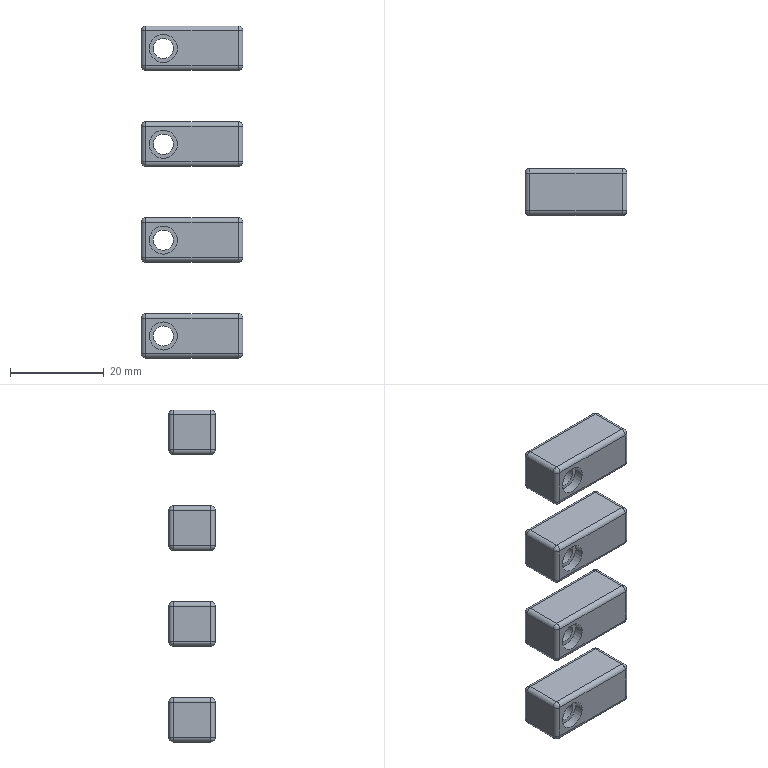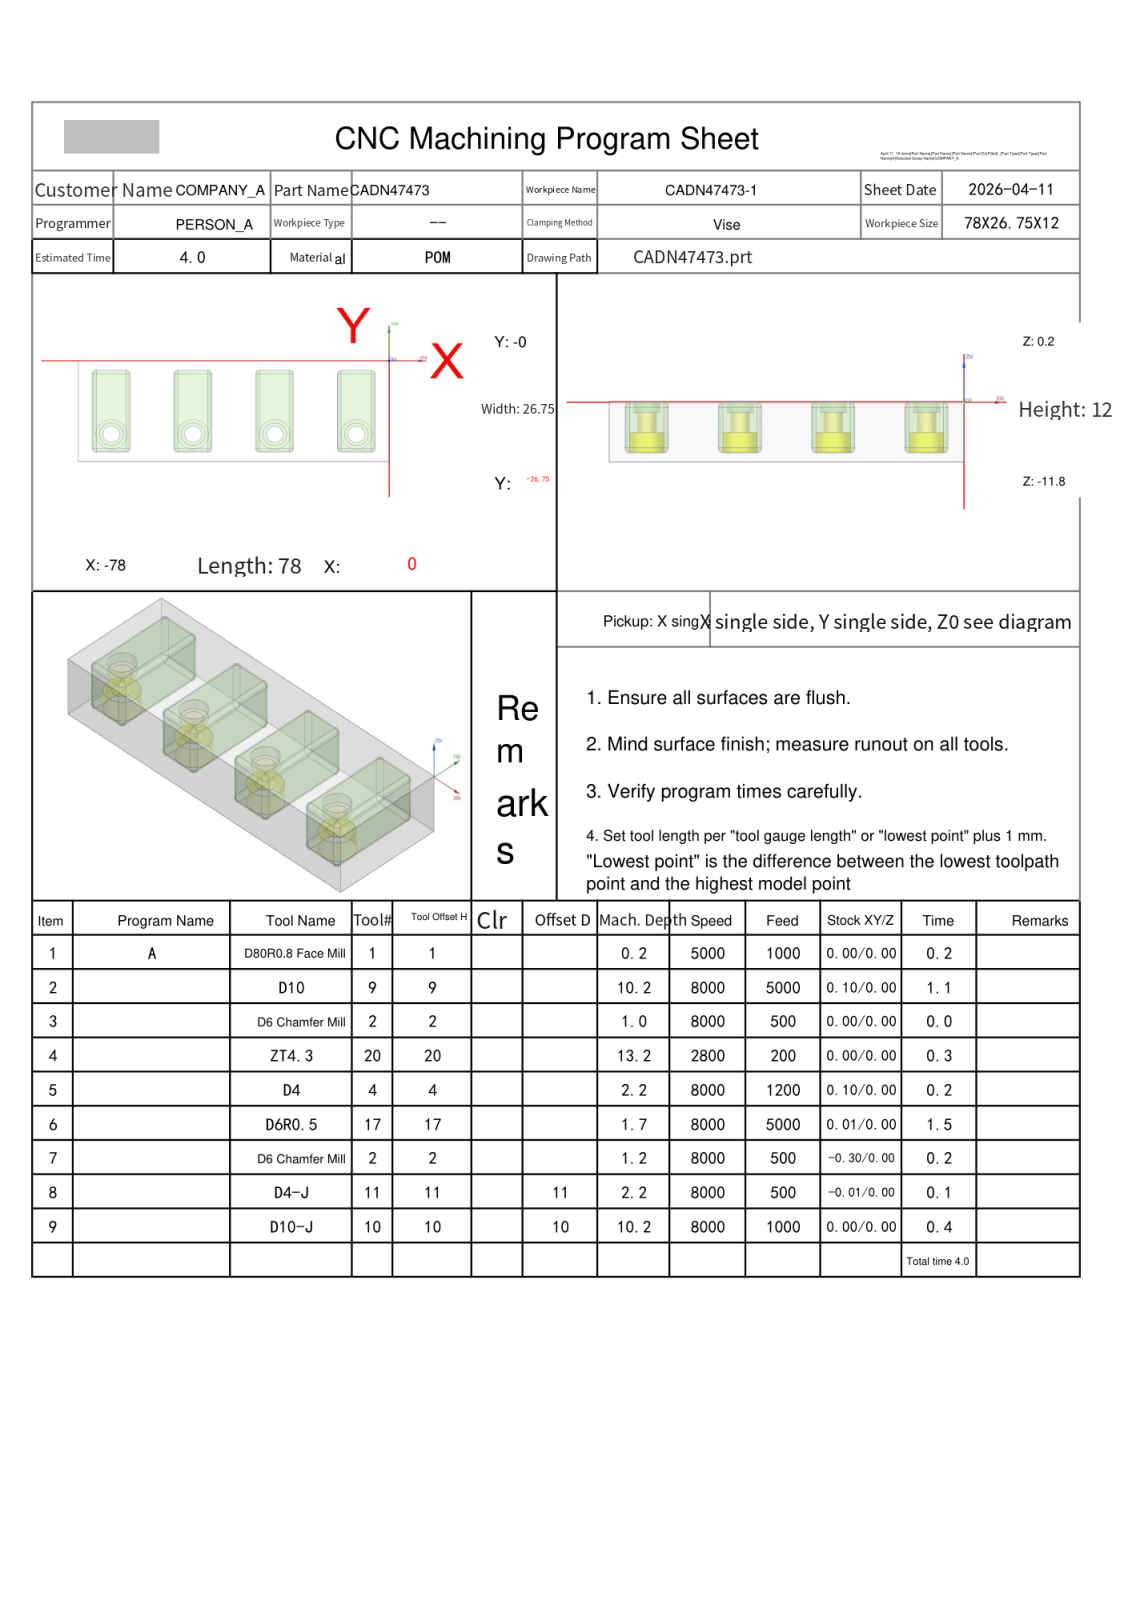NC program | NX | posted by the shop | part box 21.75 x 10 x 71 mm
Lines 681 to 1989 of 15665:
N6 T17 M06
(D6R0.5  D=6. R=0.5 H=17 ce=0.01 di=0.00)
G00 G90 G54 X-63.322 Y-10.368 M03 S8000
G43 H17 Z20.
M08
Z1.5
G01 Y-23.414 Z.816 F5000.
X-63.383 Y-23.841 Z.794
X-63.511 Y-24.253 Z.771
X-63.704 Y-24.639 Z.748
X-63.956 Y-24.989 Z.726
X-64.261 Y-25.294 Z.703
X-64.611 Y-25.546 Z.681
X-64.997 Y-25.739 Z.658
X-65.409 Y-25.867 Z.635
X-65.836 Y-25.928 Z.613
X-73.664 Z.203
X-74.091 Y-25.867 Z.18
X-74.503 Y-25.739 Z.157
X-74.889 Y-25.546 Z.135
X-75.239 Y-25.294 Z.112
X-75.544 Y-24.989 Z.09
X-75.796 Y-24.639 Z.067
X-75.989 Y-24.253 Z.044
X-76.117 Y-23.841 Z.022
X-76.178 Y-23.414 Z-.001
Y-23.25 Z-.009
Y-3.5
G02 X-73.5 Y-.822 I2.678 J0.0
G01 X-66.
G02 X-63.322 Y-3.5 I0.0 J-2.678
G01 Y-23.25
G02 X-66. Y-25.928 I-2.678 J0.0
G01 X-73.5
G02 X-76.178 Y-23.25 I0.0 J2.678
G01 X-76.181 Y-20.781 Z-.01
X-76.187 Y-18.313 Z-.011
X-76.191 Y-15.844
X-76.196 Y-13.375 Z-.012
X-76.2 Y-10.906
X-76.204 Y-8.438 Z-.013
X-76.209 Y-5.969
X-76.212 Y-3.5 Z-.014
Y-3.418
X-76.208 Y-3.336
X-76.202 Y-3.254
X-76.193 Y-3.173
X-76.183 Y-3.092
X-76.169 Y-3.011
X-76.153 Y-2.93
X-76.134 Y-2.851
X-76.114 Y-2.771
X-76.091 Y-2.693
X-76.066 Y-2.615
X-76.037 Y-2.538
X-76.008 Y-2.461
X-75.975 Y-2.386
X-75.941 Y-2.312
X-75.903 Y-2.239
X-75.865 Y-2.166
X-75.823 Y-2.096
X-75.78 Y-2.026
X-75.734 Y-1.958
X-75.687 Y-1.891
X-75.637 Y-1.826
X-75.586 Y-1.761
X-75.533 Y-1.699
X-75.478 Y-1.638
X-75.42 Y-1.58
X-75.362 Y-1.522
X-75.301 Y-1.467
X-75.239 Y-1.413
X-75.175 Y-1.362
X-75.11 Y-1.312
X-75.043 Y-1.264
X-74.975 Y-1.218
X-74.905 Y-1.175
X-74.835 Y-1.133
X-74.763 Y-1.094
X-74.69 Y-1.056
X-74.615 Y-1.022 Z-.015
X-74.54 Y-.989
X-74.464 Y-.959
X-74.387 Y-.93
X-74.309 Y-.905
X-74.23 Y-.881
X-74.15 Y-.861
X-74.071 Y-.842
X-73.99 Y-.826
X-73.909 Y-.812
X-73.828 Y-.801
X-73.746 Y-.792
X-73.664 Y-.786
X-73.582 Y-.782
X-73.5 Y-.781
X-71.625 Y-.778
X-69.75 Y-.775 Z-.016
X-67.875 Y-.772
X-66. Y-.769
X-65.918 Y-.77
X-65.835 Y-.773
X-65.753 Y-.78
X-65.671 Y-.788
X-65.589 Y-.799 Z-.017
X-65.508 Y-.813
X-65.427 Y-.829
X-65.346 Y-.847
X-65.266 Y-.868
X-65.187 Y-.891
X-65.109 Y-.917
X-65.031 Y-.945
X-64.954 Y-.975
X-64.878 Y-1.008
X-64.804 Y-1.043
X-64.73 Y-1.08
X-64.657 Y-1.119
X-64.586 Y-1.161
X-64.516 Y-1.205
X-64.447 Y-1.25
X-64.38 Y-1.298
X-64.314 Y-1.348
X-64.25 Y-1.4
X-64.187 Y-1.454
X-64.126 Y-1.509
X-64.067 Y-1.567
X-64.009 Y-1.626
X-63.953 Y-1.687
X-63.899 Y-1.749
X-63.847 Y-1.813
X-63.797 Y-1.879
X-63.749 Y-1.946
X-63.703 Y-2.015
X-63.659 Y-2.085
X-63.617 Y-2.156
X-63.578 Y-2.229
X-63.54 Y-2.302
X-63.505 Y-2.377
X-63.472 Y-2.453
X-63.442 Y-2.53
X-63.414 Y-2.607
X-63.388 Y-2.686
X-63.364 Y-2.765
X-63.343 Y-2.845
X-63.324 Y-2.926
X-63.308 Y-3.007
X-63.294 Y-3.088
X-63.283 Y-3.17
X-63.274 Y-3.252
X-63.268 Y-3.335
X-63.264 Y-3.417
X-63.263 Y-3.5
X-63.26 Y-5.969 Z-.018
X-63.256 Y-8.438
X-63.252 Y-10.906 Z-.019
X-63.249 Y-13.375 Z-.02
X-63.245 Y-15.844
X-63.243 Y-18.313 Z-.021
X-63.239 Y-20.781
X-63.236 Y-23.25 Z-.022
X-63.237 Y-23.333
X-63.241 Y-23.417
X-63.247 Y-23.5
X-63.256 Y-23.583
X-63.267 Y-23.666
X-63.28 Y-23.748
X-63.297 Y-23.83
X-63.315 Y-23.912
X-63.336 Y-23.993
X-63.36 Y-24.073
X-63.386 Y-24.152
X-63.414 Y-24.231
X-63.445 Y-24.308
X-63.478 Y-24.385
X-63.513 Y-24.461
X-63.551 Y-24.535
X-63.591 Y-24.609
X-63.633 Y-24.681
X-63.677 Y-24.752
X-63.723 Y-24.821
X-63.772 Y-24.89
X-63.822 Y-24.956
X-63.875 Y-25.021
X-63.929 Y-25.085
X-63.985 Y-25.147
X-64.043 Y-25.207
X-64.103 Y-25.265
X-64.165 Y-25.321
X-64.228 Y-25.376
X-64.293 Y-25.429
X-64.36 Y-25.479
X-64.428 Y-25.528
X-64.497 Y-25.574
X-64.568 Y-25.619
X-64.64 Y-25.661
X-64.714 Y-25.701
X-64.788 Y-25.739
X-64.864 Y-25.775
X-64.941 Y-25.808
X-65.018 Y-25.839
X-65.097 Y-25.867
X-65.176 Y-25.893 Z-.023
X-65.256 Y-25.917
X-65.337 Y-25.939
X-65.419 Y-25.957
X-65.501 Y-25.974
X-65.583 Y-25.988
X-65.666 Y-25.999
X-65.749 Y-26.008
X-65.833 Y-26.015
X-65.916 Y-26.018
X-66. Y-26.02
X-67.875 Y-26.022
X-69.75 Y-26.024 Z-.024
X-71.625 Y-26.026
X-73.5 Y-26.029
X-73.584 Y-26.028
X-73.668 Y-26.024
X-73.752 Y-26.018
X-73.835 Y-26.009
X-73.918 Y-25.998
X-74.001 Y-25.984
X-74.083 Y-25.968
X-74.165 Y-25.949
X-74.247 Y-25.928 Z-.025
X-74.327 Y-25.904
X-74.407 Y-25.878
X-74.486 Y-25.849
X-74.564 Y-25.819
X-74.641 Y-25.785
X-74.717 Y-25.75
X-74.792 Y-25.712
X-74.866 Y-25.672
X-74.938 Y-25.629
X-75.01 Y-25.585
X-75.08 Y-25.538
X-75.148 Y-25.49
X-75.215 Y-25.439
X-75.281 Y-25.387
X-75.344 Y-25.332
X-75.407 Y-25.275
X-75.467 Y-25.217
X-75.526 Y-25.157
X-75.582 Y-25.094
X-75.637 Y-25.031
X-75.69 Y-24.965
X-75.741 Y-24.899
X-75.789 Y-24.83
X-75.837 Y-24.761
X-75.881 Y-24.689
X-75.924 Y-24.617
X-75.964 Y-24.543
X-76.002 Y-24.468
X-76.037 Y-24.392
X-76.071 Y-24.315
X-76.102 Y-24.237
X-76.131 Y-24.158
X-76.157 Y-24.078
X-76.181 Y-23.997
X-76.202 Y-23.916
X-76.222 Y-23.834
X-76.238 Y-23.752
X-76.252 Y-23.669
X-76.263 Y-23.586
X-76.273 Y-23.502
X-76.279 Y-23.418
X-76.283 Y-23.334
X-76.284 Y-23.25
X-76.288 Y-20.781 Z-.026
X-76.292 Y-18.313 Z-.027
X-76.296 Y-15.844 Z-.028
X-76.3 Y-13.375
X-76.304 Y-10.906 Z-.029
X-76.308 Y-8.438 Z-.03
X-76.311 Y-5.969 Z-.031
X-76.315 Y-3.5
X-76.311 Y-3.342
X-76.298 Y-3.185 Z-.032
X-76.276 Y-3.028
X-76.245 Y-2.873
X-76.206 Y-2.72
X-76.158 Y-2.57
X-76.102 Y-2.422
X-76.038 Y-2.278
X-75.966 Y-2.137
X-75.885 Y-2.001
X-75.798 Y-1.869
X-75.703 Y-1.743
X-75.601 Y-1.622
X-75.493 Y-1.507
X-75.378 Y-1.398
X-75.257 Y-1.296
X-75.131 Y-1.201
X-75. Y-1.113
X-74.864 Y-1.032
X-74.723 Y-.96
X-74.579 Y-.895
X-74.431 Y-.838 Z-.033
X-74.281 Y-.79
X-74.128 Y-.75
X-73.973 Y-.719
X-73.816 Y-.697
X-73.658 Y-.683
X-73.5 Y-.679
X-71.625 Y-.676
X-69.75 Y-.673 Z-.034
X-67.875 Y-.67 Z-.035
X-66. Y-.667
X-65.841 Y-.672
X-65.683 Y-.685
X-65.525 Y-.707
X-65.369 Y-.737
X-65.216 Y-.777
X-65.064 Y-.825
X-64.915 Y-.882
X-64.77 Y-.946 Z-.036
X-64.629 Y-1.019
X-64.492 Y-1.1
X-64.359 Y-1.188
X-64.232 Y-1.283
X-64.111 Y-1.386
X-63.995 Y-1.495
X-63.885 Y-1.61
X-63.783 Y-1.732
X-63.687 Y-1.859
X-63.598 Y-1.991
X-63.517 Y-2.128
X-63.444 Y-2.269
X-63.379 Y-2.414
X-63.322 Y-2.563
X-63.273 Y-2.714
X-63.233 Y-2.869
X-63.202 Y-3.025
X-63.18 Y-3.182
X-63.166 Y-3.341
X-63.161 Y-3.5 Z-.037
X-63.158 Y-5.969
X-63.155 Y-8.438 Z-.038
X-63.151 Y-10.906 Z-.039
X-63.148 Y-13.375 Z-.04
X-63.145 Y-15.844
X-63.142 Y-18.313 Z-.041
X-63.139 Y-20.781 Z-.042
X-63.135 Y-23.25 Z-.043
X-63.139 Y-23.411
X-63.153 Y-23.571
X-63.175 Y-23.73
X-63.206 Y-23.888
X-63.246 Y-24.043
X-63.295 Y-24.197
X-63.352 Y-24.347
X-63.417 Y-24.494
X-63.491 Y-24.637
X-63.573 Y-24.775
X-63.662 Y-24.909
X-63.758 Y-25.038
X-63.862 Y-25.161
X-63.972 Y-25.278
X-64.089 Y-25.388
X-64.212 Y-25.492
X-64.34 Y-25.589
X-64.474 Y-25.679 Z-.044
X-64.612 Y-25.761
X-64.755 Y-25.835
X-64.902 Y-25.901
X-65.052 Y-25.958
X-65.206 Y-26.007
X-65.361 Y-26.048
X-65.519 Y-26.079
X-65.679 Y-26.102
X-65.839 Y-26.116
X-66. Y-26.121
X-67.875 Y-26.123 Z-.045
X-69.75 Y-26.125
X-71.625 Y-26.128 Z-.046
X-73.5 Y-26.13
X-73.661 Y-26.125
X-73.822 Y-26.112
X-73.982 Y-26.09 Z-.047
X-74.141 Y-26.058
X-74.298 Y-26.018
X-74.451 Y-25.969
X-74.603 Y-25.912
X-74.75 Y-25.846
X-74.894 Y-25.772
X-75.033 Y-25.69
X-75.168 Y-25.6
X-75.297 Y-25.503
X-75.421 Y-25.399
X-75.538 Y-25.288
X-75.649 Y-25.171
X-75.754 Y-25.047
X-75.851 Y-24.918
X-75.941 Y-24.784
X-76.024 Y-24.645
X-76.098 Y-24.501
X-76.164 Y-24.354
X-76.222 Y-24.202
X-76.272 Y-24.048 Z-.048
X-76.312 Y-23.892
X-76.344 Y-23.733
X-76.367 Y-23.573
X-76.381 Y-23.412
X-76.386 Y-23.25
X-76.389 Y-20.781 Z-.049
X-76.393 Y-18.313 Z-.05
X-76.396 Y-15.844 Z-.051
X-76.4 Y-13.375 Z-.052
X-76.404 Y-10.906 Z-.053
X-76.407 Y-8.438 Z-.054
X-76.41 Y-5.969 Z-.055
X-76.414 Y-3.5 Z-.056
X-76.41 Y-3.337
X-76.396 Y-3.174
X-76.374 Y-3.012
X-76.342 Y-2.851
X-76.301 Y-2.693
X-76.252 Y-2.537
X-76.194 Y-2.384
X-76.127 Y-2.235
X-76.052 Y-2.089
X-75.969 Y-1.948
X-75.879 Y-1.812
X-75.78 Y-1.681
X-75.675 Y-1.556
X-75.563 Y-1.437
X-75.444 Y-1.324 Z-.057
X-75.319 Y-1.219
X-75.189 Y-1.12
X-75.053 Y-1.029
X-74.912 Y-.946
X-74.766 Y-.87
X-74.617 Y-.803
X-74.464 Y-.745
X-74.308 Y-.695
X-74.15 Y-.654
X-73.989 Y-.621
X-73.827 Y-.598
X-73.664 Y-.584
X-73.5 Y-.58
X-71.625 Y-.577 Z-.058
X-69.75 Y-.574 Z-.059
X-67.875 Y-.572 Z-.06
X-66. Y-.569
X-65.836 Y-.573
X-65.672 Y-.587
X-65.509 Y-.61 Z-.061
X-65.348 Y-.642
X-65.188 Y-.683
X-65.031 Y-.732
X-64.878 Y-.791
X-64.727 Y-.858
X-64.581 Y-.933
X-64.439 Y-1.016
X-64.303 Y-1.108
X-64.171 Y-1.206
X-64.045 Y-1.312
X-63.925 Y-1.425
X-63.812 Y-1.545
X-63.706 Y-1.67
X-63.607 Y-1.802
X-63.515 Y-1.938 Z-.062
X-63.431 Y-2.08
X-63.355 Y-2.226
X-63.288 Y-2.377
X-63.229 Y-2.53
X-63.179 Y-2.687
X-63.137 Y-2.847
X-63.105 Y-3.008
X-63.082 Y-3.171
X-63.068 Y-3.335
X-63.063 Y-3.5
X-63.059 Y-5.969 Z-.063
X-63.056 Y-8.438 Z-.064
X-63.053 Y-10.906 Z-.065
X-63.05 Y-13.375 Z-.066
X-63.047 Y-15.844 Z-.067
X-63.044 Y-18.313 Z-.068
X-63.041 Y-20.781 Z-.069
X-63.038 Y-23.25 Z-.07
X-63.042 Y-23.416
X-63.056 Y-23.582
X-63.079 Y-23.746
X-63.111 Y-23.909
X-63.152 Y-24.07
X-63.203 Y-24.229
X-63.262 Y-24.384
X-63.329 Y-24.536
X-63.405 Y-24.684 Z-.071
X-63.49 Y-24.827
X-63.582 Y-24.966
X-63.682 Y-25.099
X-63.789 Y-25.226
X-63.903 Y-25.347
X-64.024 Y-25.461
X-64.151 Y-25.569
X-64.284 Y-25.669
X-64.422 Y-25.762
X-64.565 Y-25.846
X-64.713 Y-25.923
X-64.865 Y-25.991
X-65.02 Y-26.051
X-65.179 Y-26.101
X-65.34 Y-26.143 Z-.072
X-65.503 Y-26.176
X-65.668 Y-26.199
X-65.834 Y-26.213
X-66. Y-26.218
X-67.875 Y-26.22 Z-.073
X-69.75 Y-26.223
X-71.625 Y-26.225 Z-.074
X-73.5 Y-26.227 Z-.075
X-73.667 Y-26.223
X-73.833 Y-26.209
X-73.999 Y-26.186
X-74.163 Y-26.154
X-74.325 Y-26.112
X-74.484 Y-26.061
X-74.64 Y-26.002
X-74.793 Y-25.934
X-74.941 Y-25.858
X-75.085 Y-25.773
X-75.224 Y-25.68
X-75.358 Y-25.58 Z-.076
X-75.486 Y-25.472
X-75.607 Y-25.357
X-75.722 Y-25.236
X-75.83 Y-25.108
X-75.931 Y-24.975
X-76.024 Y-24.836
X-76.109 Y-24.692
X-76.186 Y-24.544
X-76.255 Y-24.391
X-76.314 Y-24.235
X-76.366 Y-24.076
X-76.407 Y-23.914
X-76.44 Y-23.75
X-76.464 Y-23.584
X-76.478 Y-23.417 Z-.077
X-76.483 Y-23.25
X-76.487 Y-20.781 Z-.078
X-76.49 Y-18.313 Z-.079
X-76.494 Y-15.844 Z-.08
X-76.497 Y-13.375 Z-.081
X-76.501 Y-10.906 Z-.083
X-76.504 Y-8.438 Z-.084
X-76.507 Y-5.969 Z-.085
X-76.51 Y-3.5 Z-.086
X-76.506 Y-3.331
X-76.492 Y-3.163
X-76.469 Y-2.996
X-76.436 Y-2.83
X-76.394 Y-2.666
X-76.343 Y-2.505 Z-.087
X-76.283 Y-2.347
X-76.214 Y-2.193
X-76.137 Y-2.043
X-76.051 Y-1.897
X-75.957 Y-1.756
X-75.856 Y-1.621
X-75.747 Y-1.492
X-75.631 Y-1.369
X-75.508 Y-1.253
X-75.379 Y-1.144
X-75.244 Y-1.042
X-75.104 Y-.948 Z-.088
X-74.958 Y-.861
X-74.808 Y-.784
X-74.654 Y-.714
X-74.496 Y-.654
X-74.335 Y-.602
X-74.171 Y-.56
X-74.005 Y-.526
X-73.838 Y-.503
X-73.669 Y-.488
X-73.5 Y-.483
X-71.625 Y-.481 Z-.089
X-69.75 Y-.478 Z-.09
X-67.875 Y-.476 Z-.091
X-66. Y-.473 Z-.092
X-65.83 Y-.478
X-65.661 Y-.492
X-65.493 Y-.515
X-65.326 Y-.548
X-65.162 Y-.59
X-65. Y-.642
X-64.841 Y-.702
X-64.686 Y-.771 Z-.093
X-64.535 Y-.849
X-64.388 Y-.935
X-64.247 Y-1.03
X-64.111 Y-1.131
X-63.981 Y-1.241
X-63.857 Y-1.357
X-63.741 Y-1.481
X-63.631 Y-1.611
X-63.528 Y-1.746
X-63.434 Y-1.887
X-63.347 Y-2.034
X-63.269 Y-2.185 Z-.094
X-63.199 Y-2.34
X-63.138 Y-2.499
X-63.087 Y-2.661
X-63.044 Y-2.825
X-63.011 Y-2.992
X-62.986 Y-3.16
X-62.972 Y-3.33
X-62.967 Y-3.5
X-62.964 Y-5.969 Z-.095
X-62.961 Y-8.438 Z-.097
X-62.958 Y-10.906 Z-.098
X-62.955 Y-13.375 Z-.099
X-62.951 Y-15.844 Z-.1
X-62.949 Y-18.313 Z-.101
X-62.946 Y-20.781 Z-.102
X-62.942 Y-23.25 Z-.104
X-62.947 Y-23.421
X-62.961 Y-23.592
X-62.985 Y-23.762
X-63.018 Y-23.931
X-63.061 Y-24.097
X-63.113 Y-24.26
X-63.174 Y-24.421
X-63.244 Y-24.577
X-63.322 Y-24.73
X-63.409 Y-24.878
X-63.504 Y-25.021 Z-.105
X-63.608 Y-25.158
X-63.718 Y-25.289
X-63.836 Y-25.414
X-63.961 Y-25.532
X-64.092 Y-25.643
X-64.229 Y-25.747
X-64.371 Y-25.842
X-64.519 Y-25.93
X-64.672 Y-26.009
X-64.828 Y-26.079
X-64.989 Y-26.14
X-65.152 Y-26.193
X-65.319 Y-26.236 Z-.106
X-65.487 Y-26.27
X-65.657 Y-26.294
X-65.828 Y-26.308
X-66. Y-26.313
X-67.875 Y-26.316 Z-.107
X-69.75 Y-26.318 Z-.108
X-71.625 Y-26.32 Z-.109
X-73.5 Y-26.322
X-73.672 Y-26.318 Z-.11
X-73.844 Y-26.303
X-74.015 Y-26.28
X-74.184 Y-26.246
X-74.351 Y-26.203
X-74.515 Y-26.151
X-74.676 Y-26.09
X-74.834 Y-26.02
X-74.987 Y-25.941
X-75.136 Y-25.853
X-75.279 Y-25.758
X-75.417 Y-25.654
X-75.549 Y-25.543 Z-.111
X-75.674 Y-25.424
X-75.793 Y-25.299
X-75.905 Y-25.168
X-76.009 Y-25.03
X-76.104 Y-24.887
X-76.192 Y-24.738
X-76.272 Y-24.585
X-76.342 Y-24.427
X-76.404 Y-24.266
X-76.457 Y-24.102
X-76.5 Y-23.935
X-76.534 Y-23.765 Z-.112
X-76.558 Y-23.595
X-76.573 Y-23.423
X-76.578 Y-23.25
X-76.582 Y-20.781 Z-.113
X-76.585 Y-18.313 Z-.115
X-76.588 Y-15.844 Z-.116
X-76.591 Y-13.375 Z-.117
X-76.595 Y-10.906 Z-.119
X-76.598 Y-8.438 Z-.12
X-76.601 Y-5.969 Z-.121
X-76.604 Y-3.5 Z-.123
X-76.603 Y-3.413
X-76.6 Y-3.326
X-76.594 Y-3.239
X-76.585 Y-3.152
X-76.574 Y-3.066
X-76.561 Y-2.98
X-76.545 Y-2.894
X-76.527 Y-2.809
X-76.507 Y-2.724
X-76.484 Y-2.64
X-76.459 Y-2.557
X-76.431 Y-2.474
X-76.401 Y-2.392
X-76.369 Y-2.311
X-76.335 Y-2.231 Z-.124
X-76.298 Y-2.152
X-76.26 Y-2.074
X-76.219 Y-1.997
X-76.176 Y-1.922
X-76.13 Y-1.847
X-76.083 Y-1.774
X-76.034 Y-1.702
X-75.982 Y-1.632
X-75.929 Y-1.563
X-75.874 Y-1.495
X-75.817 Y-1.43
X-75.758 Y-1.365
X-75.697 Y-1.303
X-75.635 Y-1.242
X-75.571 Y-1.183
X-75.505 Y-1.126
X-75.438 Y-1.07
X-75.369 Y-1.017
X-75.298 Y-.965
X-75.227 Y-.916
X-75.154 Y-.868 Z-.125
X-75.079 Y-.823
X-75.004 Y-.779
X-74.927 Y-.738
X-74.849 Y-.699
X-74.77 Y-.662
X-74.69 Y-.628
X-74.609 Y-.595
X-74.527 Y-.565
X-74.444 Y-.538
X-74.361 Y-.512
X-74.277 Y-.489
X-74.192 Y-.469
X-74.107 Y-.45
X-74.021 Y-.434
X-73.935 Y-.421
X-73.848 Y-.41
X-73.761 Y-.401
X-73.674 Y-.395
X-73.587 Y-.391
X-73.5 Y-.39 Z-.126
X-71.625 Y-.387 Z-.127
X-69.75 Y-.385 Z-.128
X-67.875 Y-.383 Z-.129
X-66. Y-.38 Z-.13
X-65.825 Y-.385
X-65.651 Y-.399
X-65.477 Y-.424
X-65.306 Y-.457
X-65.136 Y-.501
X-64.969 Y-.554
X-64.805 Y-.616
X-64.646 Y-.687
X-64.49 Y-.768 Z-.131
X-64.339 Y-.856
X-64.193 Y-.954
X-64.053 Y-1.059
X-63.919 Y-1.172
X-63.792 Y-1.292
X-63.671 Y-1.419
X-63.558 Y-1.552
X-63.452 Y-1.692
X-63.355 Y-1.838
X-63.266 Y-1.989 Z-.132
X-63.185 Y-2.144
X-63.113 Y-2.304
X-63.05 Y-2.468
X-62.997 Y-2.635
X-62.953 Y-2.805
X-62.919 Y-2.976
X-62.894 Y-3.15
X-62.879 Y-3.325
X-62.874 Y-3.5
X-62.871 Y-5.969 Z-.134
X-62.868 Y-8.438 Z-.135
X-62.865 Y-10.906 Z-.137
X-62.862 Y-13.375 Z-.138
X-62.859 Y-15.844 Z-.139
X-62.856 Y-18.313 Z-.141
X-62.853 Y-20.781 Z-.142
X-62.85 Y-23.25 Z-.143
X-62.851 Y-23.338
X-62.855 Y-23.427 Z-.144
X-62.861 Y-23.515
X-62.87 Y-23.603
X-62.881 Y-23.69
X-62.894 Y-23.778
X-62.91 Y-23.865
X-62.928 Y-23.951
X-62.949 Y-24.037
X-62.972 Y-24.122
X-62.998 Y-24.207
X-63.026 Y-24.291
X-63.089 Y-24.456
X-63.161 Y-24.617
X-63.242 Y-24.775
X-63.331 Y-24.927
X-63.429 Y-25.074
X-63.535 Y-25.215 Z-.145
X-63.649 Y-25.351
X-63.771 Y-25.479
X-63.899 Y-25.601
X-64.034 Y-25.715
X-64.175 Y-25.822
X-64.322 Y-25.92
X-64.474 Y-26.01
X-64.632 Y-26.092
X-64.793 Y-26.164
X-64.958 Y-26.227 Z-.146
X-65.127 Y-26.281
X-65.298 Y-26.326
X-65.472 Y-26.36
X-65.647 Y-26.385
X-65.823 Y-26.401
X-66. Y-26.406
X-67.875 Y-26.408 Z-.147
X-69.75 Y-26.41 Z-.148
X-71.625 Y-26.412 Z-.149
X-73.5 Y-26.414 Z-.15
X-73.677 Y-26.41
X-73.854 Y-26.395 Z-.151
X-74.03 Y-26.37
X-74.204 Y-26.336
X-74.376 Y-26.292
X-74.546 Y-26.238
X-74.712 Y-26.175
X-74.874 Y-26.102
X-75.032 Y-26.021
X-75.185 Y-25.931
X-75.332 Y-25.833
X-75.474 Y-25.726 Z-.152
X-75.61 Y-25.611
X-75.74 Y-25.49
X-75.862 Y-25.361
X-75.977 Y-25.225
X-76.084 Y-25.083
X-76.182 Y-24.935
X-76.273 Y-24.783
X-76.355 Y-24.625
X-76.392 Y-24.544
X-76.427 Y-24.463
X-76.46 Y-24.38
X-76.491 Y-24.297 Z-.153
X-76.519 Y-24.212
X-76.545 Y-24.127
X-76.569 Y-24.042
X-76.59 Y-23.955
X-76.608 Y-23.868
X-76.625 Y-23.781
X-76.638 Y-23.693
X-76.65 Y-23.605
X-76.665 Y-23.428
X-76.67 Y-23.25
X-76.673 Y-20.781 Z-.155
X-76.677 Y-18.313 Z-.156
X-76.68 Y-15.844 Z-.158
X-76.683 Y-13.375 Z-.159
X-76.686 Y-10.906 Z-.161
X-76.689 Y-8.438 Z-.162
X-76.692 Y-5.969 Z-.164
X-76.695 Y-3.5 Z-.166
X-76.694 Y-3.41
X-76.69 Y-3.321
X-76.684 Y-3.231
X-76.675 Y-3.142
X-76.664 Y-3.053
X-76.65 Y-2.965
X-76.634 Y-2.877
X-76.616 Y-2.789
X-76.595 Y-2.702
X-76.571 Y-2.615
X-76.545 Y-2.529
X-76.517 Y-2.444
X-76.486 Y-2.36
X-76.453 Y-2.277
X-76.418 Y-2.194
X-76.38 Y-2.113 Z-.167
X-76.34 Y-2.033
X-76.298 Y-1.954
X-76.254 Y-1.876
X-76.207 Y-1.799
X-76.159 Y-1.724
X-76.108 Y-1.65
X-76.055 Y-1.577
X-76. Y-1.506
X-75.943 Y-1.437
X-75.884 Y-1.369
X-75.824 Y-1.303
X-75.761 Y-1.239
X-75.697 Y-1.176
X-75.631 Y-1.115
X-75.564 Y-1.056
X-75.494 Y-.999
X-75.423 Y-.944
X-75.351 Y-.891 Z-.168
X-75.277 Y-.84
X-75.202 Y-.791
X-75.125 Y-.745
X-75.047 Y-.7
X-74.968 Y-.658
X-74.888 Y-.618
X-74.807 Y-.579
X-74.724 Y-.544
X-74.641 Y-.511
X-74.557 Y-.48
X-74.472 Y-.451
X-74.386 Y-.425
X-74.299 Y-.401
X-74.212 Y-.38
X-74.124 Y-.361
X-74.036 Y-.345
X-73.947 Y-.331 Z-.169
X-73.858 Y-.32
X-73.769 Y-.31
X-73.679 Y-.304
X-73.59 Y-.3
X-73.5 Y-.299
X-71.625 Y-.296 Z-.17
X-69.75 Y-.294 Z-.171
X-67.875 Y-.292 Z-.172
X-66. Y-.29 Z-.174
X-65.91 Y-.291
X-65.82 Y-.295
X-65.73 Y-.301
X-65.641 Y-.31
X-65.551 Y-.321
X-65.462 Y-.334
X-65.374 Y-.351
X-65.285 Y-.369
X-65.198 Y-.391
X-65.111 Y-.414
X-65.025 Y-.44
X-64.939 Y-.469
X-64.855 Y-.499
X-64.771 Y-.533
X-64.688 Y-.568
X-64.606 Y-.606
X-64.526 Y-.646 Z-.175
X-64.446 Y-.689
X-64.368 Y-.733
X-64.291 Y-.78
X-64.215 Y-.829
X-64.141 Y-.88
X-64.068 Y-.933
X-63.997 Y-.988
X-63.927 Y-1.045
X-63.859 Y-1.104
X-63.793 Y-1.165
X-63.728 Y-1.228
X-63.665 Y-1.292
X-63.604 Y-1.359
X-63.545 Y-1.427
X-63.487 Y-1.496
X-63.432 Y-1.567
X-63.379 Y-1.64
X-63.328 Y-1.714 Z-.176
X-63.278 Y-1.79
X-63.232 Y-1.867
X-63.187 Y-1.945
X-63.144 Y-2.025
X-63.104 Y-2.105
X-63.066 Y-2.187
X-63.03 Y-2.27
X-62.996 Y-2.353
X-62.965 Y-2.438
X-62.937 Y-2.524
X-62.91 Y-2.61
X-62.887 Y-2.697
X-62.865 Y-2.784
X-62.846 Y-2.873
X-62.83 Y-2.961
X-62.816 Y-3.05
X-62.804 Y-3.14
X-62.795 Y-3.23 Z-.177
X-62.789 Y-3.32
X-62.785 Y-3.41
X-62.784 Y-3.5
X-62.781 Y-5.969 Z-.178
X-62.778 Y-8.438 Z-.18
X-62.775 Y-10.906 Z-.181
X-62.772 Y-13.375 Z-.183
X-62.769 Y-15.844 Z-.185
X-62.767 Y-18.313 Z-.186
X-62.764 Y-20.781 Z-.188
X-62.761 Y-23.25 Z-.189
X-62.762 Y-23.341
X-62.766 Y-23.432
X-62.772 Y-23.522
X-62.781 Y-23.613
X-62.792 Y-23.703 Z-.19
X-62.806 Y-23.793
X-62.822 Y-23.882
X-62.841 Y-23.971
X-62.863 Y-24.059
X-62.887 Y-24.147
X-62.913 Y-24.234
X-62.942 Y-24.32
X-62.973 Y-24.406
X-63.006 Y-24.49
X-63.042 Y-24.574
X-63.08 Y-24.656
X-63.121 Y-24.738
X-63.163 Y-24.818
X-63.208 Y-24.897
X-63.256 Y-24.974
X-63.305 Y-25.051
X-63.356 Y-25.126
X-63.41 Y-25.199 Z-.191
X-63.466 Y-25.271
X-63.523 Y-25.342
X-63.583 Y-25.41
X-63.644 Y-25.477
X-63.708 Y-25.542
X-63.773 Y-25.606
X-63.84 Y-25.667
X-63.908 Y-25.727
X-63.978 Y-25.785
X-64.05 Y-25.841
X-64.124 Y-25.895
X-64.198 Y-25.946
X-64.275 Y-25.996
X-64.352 Y-26.043
X-64.431 Y-26.088
X-64.511 Y-26.131
X-64.593 Y-26.172 Z-.192
X-64.675 Y-26.211
X-64.759 Y-26.247
X-64.843 Y-26.28
X-64.929 Y-26.312
X-65.015 Y-26.341
X-65.102 Y-26.367
X-65.19 Y-26.391
X-65.278 Y-26.413
X-65.367 Y-26.432
X-65.457 Y-26.448
X-65.546 Y-26.463
X-65.637 Y-26.474
X-65.727 Y-26.483
X-65.818 Y-26.49
X-65.909 Y-26.494
X-66. Y-26.495
X-67.875 Y-26.497 Z-.194
X-69.75 Y-26.499 Z-.195
X-71.625 Y-26.501 Z-.196
X-73.5 Y-26.503 Z-.197
X-73.591 Y-26.502
X-73.682 Y-26.498
X-73.773 Y-26.492
X-73.864 Y-26.483
X-73.955 Y-26.472
X-74.045 Y-26.458 Z-.198
X-74.135 Y-26.442
X-74.224 Y-26.423
X-74.313 Y-26.401
X-74.401 Y-26.377
X-74.488 Y-26.351
X-74.575 Y-26.322
X-74.661 Y-26.291
X-74.746 Y-26.257
X-74.829 Y-26.221
X-74.912 Y-26.183
X-74.994 Y-26.142
X-75.075 Y-26.099
X-75.154 Y-26.054
X-75.232 Y-26.006
X-75.309 Y-25.957
X-75.384 Y-25.905
X-75.458 Y-25.851 Z-.199
X-75.53 Y-25.795
X-75.601 Y-25.738
X-75.67 Y-25.678
X-75.737 Y-25.616
X-75.802 Y-25.552
X-75.866 Y-25.487
X-75.928 Y-25.42
X-75.988 Y-25.351
X-76.046 Y-25.28
X-76.102 Y-25.208
X-76.156 Y-25.135
X-76.208 Y-25.059
X-76.258 Y-24.983
X-76.305 Y-24.905
X-76.351 Y-24.826
X-76.394 Y-24.745
X-76.435 Y-24.663
X-76.473 Y-24.581 Z-.2
X-76.51 Y-24.497
X-76.544 Y-24.412
X-76.575 Y-24.326
X-76.604 Y-24.239
X-76.631 Y-24.152
X-76.655 Y-24.064
X-76.676 Y-23.975
X-76.696 Y-23.886
X-76.712 Y-23.796
X-76.727 Y-23.706
X-76.738 Y-23.615
X-76.747 Y-23.524
X-76.754 Y-23.433
X-76.758 Y-23.341
X-76.759 Y-23.25
X-76.762 Y-20.781 Z-.202
X-76.765 Y-18.313 Z-.204
X-76.768 Y-15.844 Z-.206
X-76.771 Y-13.375 Z-.207
X-76.774 Y-10.906 Z-.209
X-76.777 Y-8.438 Z-.211
X-76.779 Y-5.969 Z-.213
X-76.782 Y-3.5 Z-.214
X-76.778 Y-3.328
X-76.765 Y-3.157 Z-.215
X-76.743 Y-2.986
X-76.711 Y-2.817
X-76.672 Y-2.65
X-76.623 Y-2.485
X-76.566 Y-2.323
X-76.5 Y-2.164
X-76.426 Y-2.009
X-76.344 Y-1.858 Z-.216
X-76.255 Y-1.711
X-76.157 Y-1.569
X-76.053 Y-1.433
X-75.941 Y-1.302
X-75.823 Y-1.177
X-75.699 Y-1.058
X-75.568 Y-.946
X-75.431 Y-.842 Z-.217
X-75.29 Y-.744
X-75.143 Y-.654
X-74.992 Y-.571
X-74.837 Y-.497
X-74.678 Y-.431
X-74.516 Y-.374
X-74.351 Y-.324
X-74.184 Y-.284
X-74.014 Y-.253 Z-.218
X-73.844 Y-.23
X-73.672 Y-.216
X-73.5 Y-.212
X-71.625 Y-.209 Z-.219
X-69.75 Y-.207 Z-.221
X-67.875 Y-.205 Z-.222
X-66. Y-.203 Z-.223
X-65.827 Y-.207
X-65.655 Y-.22 Z-.224
X-65.484 Y-.243
X-65.314 Y-.274
X-65.146 Y-.314
X-64.981 Y-.363
X-64.818 Y-.421
X-64.658 Y-.486
X-64.502 Y-.561
X-64.35 Y-.643
X-64.203 Y-.733 Z-.225
X-64.061 Y-.831
X-63.923 Y-.936
X-63.792 Y-1.048
X-63.666 Y-1.166
X-63.547 Y-1.292
X-63.435 Y-1.423
X-63.33 Y-1.56
X-63.232 Y-1.702 Z-.226
X-63.141 Y-1.849
X-63.058 Y-2.001
X-62.984 Y-2.157
X-62.918 Y-2.317
X-62.86 Y-2.48
X-62.81 Y-2.645
X-62.77 Y-2.813
X-62.738 Y-2.983 Z-.227
X-62.715 Y-3.155
X-62.702 Y-3.327
X-62.697 Y-3.5
X-62.694 Y-5.969 Z-.229
X-62.691 Y-8.438 Z-.23
X-62.689 Y-10.906 Z-.232
X-62.686 Y-13.375 Z-.234
X-62.683 Y-15.844 Z-.236
X-62.681 Y-18.313 Z-.237
X-62.678 Y-20.781 Z-.239
X-62.675 Y-23.25 Z-.241
X-62.679 Y-23.424
X-62.693 Y-23.598
X-62.715 Y-23.77
X-62.747 Y-23.941
X-62.787 Y-24.111
X-62.837 Y-24.278 Z-.242
X-62.895 Y-24.442
X-62.961 Y-24.603
X-63.036 Y-24.76
X-63.119 Y-24.913
X-63.21 Y-25.062
X-63.308 Y-25.206
X-63.414 Y-25.344
X-63.527 Y-25.477 Z-.243
X-63.647 Y-25.603
X-63.773 Y-25.723
X-63.906 Y-25.837
X-64.044 Y-25.943
X-64.187 Y-26.042
X-64.336 Y-26.133
X-64.489 Y-26.216
X-64.646 Y-26.291 Z-.244
X-64.807 Y-26.358
X-64.971 Y-26.417
X-65.138 Y-26.466
X-65.308 Y-26.507
X-65.479 Y-26.539
X-65.652 Y-26.562
X-65.826 Y-26.576
X-66. Y-26.581 Z-.245
X-67.875 Y-26.583 Z-.246
X-69.75 Y-26.585 Z-.247
X-71.625 Y-26.587 Z-.248
X-73.5 Y-26.589 Z-.25
X-73.675 Y-26.584
X-73.849 Y-26.571
X-74.022 Y-26.548
X-74.194 Y-26.517
X-74.364 Y-26.476
X-74.532 Y-26.426 Z-.251
X-74.697 Y-26.368
X-74.859 Y-26.301
X-75.016 Y-26.226
X-75.17 Y-26.143
X-75.319 Y-26.052
X-75.464 Y-25.953
X-75.603 Y-25.847
X-75.736 Y-25.733 Z-.252
X-75.863 Y-25.613
X-75.983 Y-25.486
X-76.097 Y-25.353
X-76.204 Y-25.214
X-76.303 Y-25.07
X-76.395 Y-24.921
X-76.478 Y-24.767
X-76.554 Y-24.61 Z-.253
X-76.621 Y-24.448
X-76.68 Y-24.283
X-76.729 Y-24.115
X-76.77 Y-23.945
X-76.803 Y-23.773
X-76.826 Y-23.6
X-76.839 Y-23.425
X-76.844 Y-23.25
X-76.847 Y-20.781 Z-.255
X-76.85 Y-18.313 Z-.257
X-76.852 Y-15.844 Z-.259
X-76.856 Y-13.375 Z-.261
X-76.858 Y-10.906 Z-.263
X-76.861 Y-8.438 Z-.265
X-76.864 Y-5.969 Z-.267
X-76.866 Y-3.5 Z-.269
X-76.862 Y-3.324
X-76.848 Y-3.148
X-76.826 Y-2.973
X-76.794 Y-2.8
X-76.753 Y-2.628
X-76.703 Y-2.459 Z-.27
X-76.644 Y-2.293
X-76.577 Y-2.13
X-76.501 Y-1.971
X-76.417 Y-1.816
X-76.325 Y-1.665
X-76.225 Y-1.52
X-76.118 Y-1.38 Z-.271
X-76.004 Y-1.246
X-75.883 Y-1.117
X-75.755 Y-.996
X-75.621 Y-.881
X-75.481 Y-.774
X-75.336 Y-.673
X-75.185 Y-.581
X-75.03 Y-.497 Z-.272
X-74.871 Y-.421
X-74.708 Y-.353
X-74.542 Y-.294
X-74.373 Y-.243
X-74.201 Y-.202
X-74.027 Y-.17
X-73.852 Y-.147 Z-.273
X-73.676 Y-.132
X-73.5 Y-.128
X-71.625 Y-.126 Z-.274
X-69.75 Y-.123 Z-.276
X-67.875 Y-.121 Z-.277
X-66. Y-.119 Z-.279
X-65.823 Y-.124
X-65.647 Y-.137
X-65.471 Y-.16
X-65.297 Y-.192
X-65.125 Y-.234
X-64.955 Y-.284
X-64.788 Y-.343 Z-.28
X-64.624 Y-.41
X-64.464 Y-.486
X-64.309 Y-.571
X-64.158 Y-.663
X-64.012 Y-.763
X-63.871 Y-.871
X-63.736 Y-.986 Z-.281
X-63.608 Y-1.108
X-63.485 Y-1.236
X-63.37 Y-1.37
X-63.262 Y-1.511
X-63.162 Y-1.657
X-63.069 Y-1.808
X-62.984 Y-1.963 Z-.282
X-62.908 Y-2.123
X-62.84 Y-2.287
X-62.78 Y-2.454